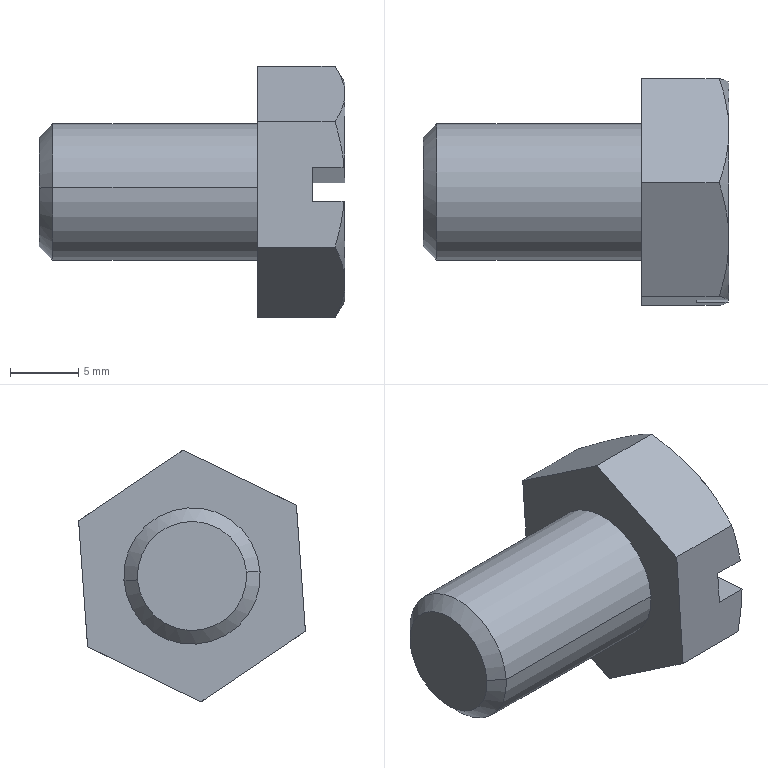Part | SolidWorks | features BaseBody 1 | 1 solid | 23 faces | box 22.4 x 16.618 x 18.428 mm | volume 2560 mm3 | plane 13 | cone 8 | cylinder 2 | commonest cylinder face diameters 10 x2
STEP:
#1=CARTESIAN_POINT('',(442.1,141.01,-29.715));
#2=VERTEX_POINT('',#1);
#3=CARTESIAN_POINT('',(442.1,148.99,-30.285));
#4=VERTEX_POINT('',#3);
#5=CARTESIAN_POINT('',(442.1,145.,-30.));
#6=DIRECTION('',(-1.,0.,0.));
#7=DIRECTION('',(0.,-0.9975,0.07126));
#8=AXIS2_PLACEMENT_3D('',#5,#6,#7);
#9=CIRCLE('',#8,4.);
#10=EDGE_CURVE('',#2,#4,#9,.T.);
#11=ORIENTED_EDGE('',*,*,#10,.F.);
#12=CARTESIAN_POINT('',(443.1,140.013,-29.644));
#13=VERTEX_POINT('',#12);
#14=CARTESIAN_POINT('',(442.1,141.01,-29.715));
#15=DIRECTION('',(0.7071,-0.7053,0.05039));
#16=VECTOR('',#15,1000.);
#17=LINE('',#14,#16);
#18=EDGE_CURVE('',#2,#13,#17,.T.);
#19=ORIENTED_EDGE('',*,*,#18,.T.);
#20=CARTESIAN_POINT('',(443.1,149.987,-30.356));
#21=VERTEX_POINT('',#20);
#22=CARTESIAN_POINT('',(443.1,145.,-30.));
#23=DIRECTION('',(1.,0.,0.));
#24=DIRECTION('',(0.,-0.9975,0.07126));
#25=AXIS2_PLACEMENT_3D('',#22,#23,#24);
#26=CIRCLE('',#25,5.);
#27=EDGE_CURVE('',#21,#13,#26,.T.);
#28=ORIENTED_EDGE('',*,*,#27,.F.);
#29=CARTESIAN_POINT('',(442.1,148.99,-30.285));
#30=DIRECTION('',(0.7071,0.7053,-0.05039));
#31=VECTOR('',#30,1000.);
#32=LINE('',#29,#31);
#33=EDGE_CURVE('',#4,#21,#32,.T.);
#34=ORIENTED_EDGE('',*,*,#33,.F.);
#35=EDGE_LOOP('',(#11,#19,#28,#34));
#36=FACE_OUTER_BOUND('',#35,.T.);
#37=CARTESIAN_POINT('',(442.1,145.,-30.));
#38=DIRECTION('',(1.,0.,0.));
#39=DIRECTION('',(0.,0.9975,-0.07126));
#40=AXIS2_PLACEMENT_3D('',#37,#38,#39);
#41=CONICAL_SURFACE('',#40,4.,0.7854);
#42=ADVANCED_FACE('',(#36),#41,.T.);
#43=ORIENTED_EDGE('',*,*,#27,.T.);
#44=CARTESIAN_POINT('',(458.1,140.013,-29.644));
#45=VERTEX_POINT('',#44);
#46=CARTESIAN_POINT('',(442.1,140.013,-29.644));
#47=DIRECTION('',(1.,0.,0.));
#48=VECTOR('',#47,1000.);
#49=LINE('',#46,#48);
#50=EDGE_CURVE('',#13,#45,#49,.T.);
#51=ORIENTED_EDGE('',*,*,#50,.T.);
#52=CARTESIAN_POINT('',(458.1,149.987,-30.356));
#53=VERTEX_POINT('',#52);
#54=CARTESIAN_POINT('',(458.1,145.,-30.));
#55=DIRECTION('',(-1.,0.,0.));
#56=DIRECTION('',(0.,-0.9975,0.07126));
#57=AXIS2_PLACEMENT_3D('',#54,#55,#56);
#58=CIRCLE('',#57,5.);
#59=EDGE_CURVE('',#45,#53,#58,.T.);
#60=ORIENTED_EDGE('',*,*,#59,.T.);
#61=CARTESIAN_POINT('',(442.1,149.987,-30.356));
#62=DIRECTION('',(1.,0.,0.));
#63=VECTOR('',#62,1000.);
#64=LINE('',#61,#63);
#65=EDGE_CURVE('',#21,#53,#64,.T.);
#66=ORIENTED_EDGE('',*,*,#65,.F.);
#67=EDGE_LOOP('',(#43,#51,#60,#66));
#68=FACE_OUTER_BOUND('',#67,.T.);
#69=CARTESIAN_POINT('',(442.1,145.,-30.));
#70=DIRECTION('',(1.,0.,0.));
#71=DIRECTION('',(0.,0.9975,-0.07126));
#72=AXIS2_PLACEMENT_3D('',#69,#70,#71);
#73=CYLINDRICAL_SURFACE('',#72,5.);
#74=ADVANCED_FACE('',(#68),#73,.T.);
#75=CARTESIAN_POINT('',(458.1,145.658,-20.786));
#76=VERTEX_POINT('',#75);
#77=CARTESIAN_POINT('',(458.1,153.309,-25.963));
#78=VERTEX_POINT('',#77);
#79=CARTESIAN_POINT('',(458.1,153.309,-25.963));
#80=DIRECTION('',(0.,0.8282,-0.5604));
#81=VECTOR('',#80,1000.);
#82=LINE('',#79,#81);
#83=EDGE_CURVE('',#76,#78,#82,.T.);
#84=ORIENTED_EDGE('',*,*,#83,.T.);
#85=CARTESIAN_POINT('',(458.1,152.651,-35.177));
#86=VERTEX_POINT('',#85);
#87=CARTESIAN_POINT('',(458.1,152.651,-35.177));
#88=DIRECTION('',(0.,-0.07126,-0.9975));
#89=VECTOR('',#88,1000.);
#90=LINE('',#87,#89);
#91=EDGE_CURVE('',#78,#86,#90,.T.);
#92=ORIENTED_EDGE('',*,*,#91,.T.);
#93=CARTESIAN_POINT('',(458.1,144.342,-39.214));
#94=VERTEX_POINT('',#93);
#95=CARTESIAN_POINT('',(458.1,152.651,-35.177));
#96=DIRECTION('',(0.,-0.8995,-0.437));
#97=VECTOR('',#96,1000.);
#98=LINE('',#95,#97);
#99=EDGE_CURVE('',#86,#94,#98,.T.);
#100=ORIENTED_EDGE('',*,*,#99,.T.);
#101=CARTESIAN_POINT('',(458.1,136.691,-34.037));
#102=VERTEX_POINT('',#101);
#103=CARTESIAN_POINT('',(458.1,136.691,-34.037));
#104=DIRECTION('',(0.,-0.8282,0.5604));
#105=VECTOR('',#104,1000.);
#106=LINE('',#103,#105);
#107=EDGE_CURVE('',#94,#102,#106,.T.);
#108=ORIENTED_EDGE('',*,*,#107,.T.);
#109=CARTESIAN_POINT('',(458.1,137.349,-24.823));
#110=VERTEX_POINT('',#109);
#111=CARTESIAN_POINT('',(458.1,136.691,-34.037));
#112=DIRECTION('',(0.,0.07126,0.9975));
#113=VECTOR('',#112,1000.);
#114=LINE('',#111,#113);
#115=EDGE_CURVE('',#102,#110,#114,.T.);
#116=ORIENTED_EDGE('',*,*,#115,.T.);
#117=CARTESIAN_POINT('',(458.1,137.349,-24.823));
#118=DIRECTION('',(0.,0.8995,0.437));
#119=VECTOR('',#118,1000.);
#120=LINE('',#117,#119);
#121=EDGE_CURVE('',#110,#76,#120,.T.);
#122=ORIENTED_EDGE('',*,*,#121,.T.);
#123=EDGE_LOOP('',(#84,#92,#100,#108,#116,#122));
#124=FACE_OUTER_BOUND('',#123,.T.);
#125=CARTESIAN_POINT('',(458.1,145.,-30.));
#126=DIRECTION('',(-1.,0.,0.));
#127=DIRECTION('',(0.,-0.9975,0.07126));
#128=AXIS2_PLACEMENT_3D('',#125,#126,#127);
#129=CIRCLE('',#128,5.);
#130=EDGE_CURVE('',#53,#45,#129,.T.);
#131=ORIENTED_EDGE('',*,*,#130,.F.);
#132=ORIENTED_EDGE('',*,*,#59,.F.);
#133=EDGE_LOOP('',(#131,#132));
#134=FACE_BOUND('',#133,.T.);
#135=CARTESIAN_POINT('',(458.1,145.658,-20.786));
#136=DIRECTION('',(-1.,0.,0.));
#137=DIRECTION('',(0.,-0.9975,0.07126));
#138=AXIS2_PLACEMENT_3D('',#135,#136,#137);
#139=PLANE('',#138);
#140=ADVANCED_FACE('',(#124,#134),#139,.T.);
#141=CARTESIAN_POINT('',(464.5,148.496,-37.196));
#142=VERTEX_POINT('',#141);
#143=CARTESIAN_POINT('',(464.5,152.793,-31.81));
#144=VERTEX_POINT('',#143);
#145=CARTESIAN_POINT('',(464.5,145.,-30.));
#146=DIRECTION('',(1.,0.,0.));
#147=DIRECTION('',(0.,0.9975,-0.07126));
#148=AXIS2_PLACEMENT_3D('',#145,#146,#147);
#149=CIRCLE('',#148,8.);
#150=EDGE_CURVE('',#142,#144,#149,.T.);
#151=ORIENTED_EDGE('',*,*,#150,.T.);
#152=CARTESIAN_POINT('',(464.5,137.029,-30.684));
#153=VERTEX_POINT('',#152);
#154=CARTESIAN_POINT('',(464.5,136.931,-30.677));
#155=DIRECTION('',(0.,0.9975,-0.07126));
#156=VECTOR('',#155,1000.);
#157=LINE('',#154,#156);
#158=EDGE_CURVE('',#153,#144,#157,.T.);
#159=ORIENTED_EDGE('',*,*,#158,.F.);
#160=CARTESIAN_POINT('',(464.5,140.516,-36.626));
#161=VERTEX_POINT('',#160);
#162=CARTESIAN_POINT('',(464.5,145.,-30.));
#163=DIRECTION('',(1.,0.,0.));
#164=DIRECTION('',(0.,0.9975,-0.07126));
#165=AXIS2_PLACEMENT_3D('',#162,#163,#164);
#166=CIRCLE('',#165,8.);
#167=EDGE_CURVE('',#153,#161,#166,.T.);
#168=ORIENTED_EDGE('',*,*,#167,.T.);
#169=CARTESIAN_POINT('',(464.5,145.,-30.));
#170=DIRECTION('',(1.,0.,0.));
#171=DIRECTION('',(0.,0.9975,-0.07126));
#172=AXIS2_PLACEMENT_3D('',#169,#170,#171);
#173=CIRCLE('',#172,8.);
#174=EDGE_CURVE('',#161,#142,#173,.T.);
#175=ORIENTED_EDGE('',*,*,#174,.T.);
#176=EDGE_LOOP('',(#151,#159,#168,#175));
#177=FACE_OUTER_BOUND('',#176,.T.);
#178=CARTESIAN_POINT('',(464.5,145.658,-20.786));
#179=DIRECTION('',(-1.,0.,0.));
#180=DIRECTION('',(0.,-0.9975,0.07126));
#181=AXIS2_PLACEMENT_3D('',#178,#179,#180);
#182=PLANE('',#181);
#183=ADVANCED_FACE('',(#177),#182,.F.);
#184=CARTESIAN_POINT('',(463.785,153.309,-25.963));
#185=VERTEX_POINT('',#184);
#186=CARTESIAN_POINT('',(464.5,149.484,-23.374));
#187=VERTEX_POINT('',#186);
#188=CARTESIAN_POINT('',(463.785,153.309,-25.963));
#189=CARTESIAN_POINT('',(464.004,152.683,-25.54));
#190=CARTESIAN_POINT('',(464.183,152.053,-25.113));
#191=CARTESIAN_POINT('',(464.432,150.779,-24.251));
#192=CARTESIAN_POINT('',(464.5,150.135,-23.815));
#193=CARTESIAN_POINT('',(464.5,149.484,-23.374));
#194=B_SPLINE_CURVE_WITH_KNOTS('',3,(#188,#189,#190,#191,#192,#193),.UNSPECIFIED.,.F.,.F.,(4,2,4),(0.000000238,0.002337,0.004674),.UNSPECIFIED.);
#195=EDGE_CURVE('',#185,#187,#194,.T.);
#196=ORIENTED_EDGE('',*,*,#195,.F.);
#197=CARTESIAN_POINT('',(458.1,153.309,-25.963));
#198=DIRECTION('',(1.,0.,0.));
#199=VECTOR('',#198,1000.);
#200=LINE('',#197,#199);
#201=EDGE_CURVE('',#78,#185,#200,.T.);
#202=ORIENTED_EDGE('',*,*,#201,.F.);
#203=ORIENTED_EDGE('',*,*,#83,.F.);
#204=CARTESIAN_POINT('',(463.785,145.658,-20.786));
#205=VERTEX_POINT('',#204);
#206=CARTESIAN_POINT('',(458.1,145.658,-20.786));
#207=DIRECTION('',(1.,0.,0.));
#208=VECTOR('',#207,1000.);
#209=LINE('',#206,#208);
#210=EDGE_CURVE('',#76,#205,#209,.T.);
#211=ORIENTED_EDGE('',*,*,#210,.T.);
#212=CARTESIAN_POINT('',(464.5,149.484,-23.374));
#213=CARTESIAN_POINT('',(464.5,149.159,-23.155));
#214=CARTESIAN_POINT('',(464.483,148.833,-22.934));
#215=CARTESIAN_POINT('',(464.418,148.188,-22.498));
#216=CARTESIAN_POINT('',(464.369,147.867,-22.281));
#217=CARTESIAN_POINT('',(464.183,146.912,-21.634));
#218=CARTESIAN_POINT('',(464.003,146.282,-21.208));
#219=CARTESIAN_POINT('',(463.785,145.658,-20.786));
#220=B_SPLINE_CURVE_WITH_KNOTS('',3,(#212,#213,#214,#215,#216,#217,#218,#219),.UNSPECIFIED.,.F.,.F.,(4,2,2,4),(0.004674,0.005838,0.007002,0.00933),.UNSPECIFIED.);
#221=EDGE_CURVE('',#187,#205,#220,.T.);
#222=ORIENTED_EDGE('',*,*,#221,.F.);
#223=EDGE_LOOP('',(#196,#202,#203,#211,#222));
#224=FACE_OUTER_BOUND('',#223,.T.);
#225=CARTESIAN_POINT('',(458.1,153.309,-25.963));
#226=DIRECTION('',(0.,-0.5604,-0.8282));
#227=DIRECTION('',(0.,-0.8282,0.5604));
#228=AXIS2_PLACEMENT_3D('',#225,#226,#227);
#229=PLANE('',#228);
#230=ADVANCED_FACE('',(#224),#229,.F.);
#231=CARTESIAN_POINT('',(463.785,152.651,-35.177));
#232=VERTEX_POINT('',#231);
#233=CARTESIAN_POINT('',(464.444,152.891,-31.817));
#234=VERTEX_POINT('',#233);
#235=CARTESIAN_POINT('',(463.785,152.651,-35.177));
#236=CARTESIAN_POINT('',(463.945,152.69,-34.628));
#237=CARTESIAN_POINT('',(464.085,152.73,-34.068));
#238=CARTESIAN_POINT('',(464.309,152.81,-32.947));
#239=CARTESIAN_POINT('',(464.393,152.85,-32.383));
#240=CARTESIAN_POINT('',(464.444,152.891,-31.817));
#241=B_SPLINE_CURVE_WITH_KNOTS('',3,(#235,#236,#237,#238,#239,#240),.UNSPECIFIED.,.F.,.F.,(4,2,4),(0.008618,0.01033,0.01204),.UNSPECIFIED.);
#242=EDGE_CURVE('',#232,#234,#241,.T.);
#243=ORIENTED_EDGE('',*,*,#242,.F.);
#244=CARTESIAN_POINT('',(458.1,152.651,-35.177));
#245=DIRECTION('',(1.,0.,0.));
#246=VECTOR('',#245,1000.);
#247=LINE('',#244,#246);
#248=EDGE_CURVE('',#86,#232,#247,.T.);
#249=ORIENTED_EDGE('',*,*,#248,.F.);
#250=ORIENTED_EDGE('',*,*,#91,.F.);
#251=ORIENTED_EDGE('',*,*,#201,.T.);
#252=CARTESIAN_POINT('',(464.444,153.069,-29.323));
#253=VERTEX_POINT('',#252);
#254=CARTESIAN_POINT('',(464.444,153.069,-29.323));
#255=CARTESIAN_POINT('',(464.341,153.151,-28.173));
#256=CARTESIAN_POINT('',(464.102,153.231,-27.058));
#257=CARTESIAN_POINT('',(463.785,153.309,-25.963));
#258=B_SPLINE_CURVE_WITH_KNOTS('',3,(#254,#255,#256,#257),.UNSPECIFIED.,.F.,.F.,(4,4),(0.01454,0.01797),.UNSPECIFIED.);
#259=EDGE_CURVE('',#253,#185,#258,.T.);
#260=ORIENTED_EDGE('',*,*,#259,.F.);
#261=CARTESIAN_POINT('',(462.1,153.069,-29.323));
#262=VERTEX_POINT('',#261);
#263=CARTESIAN_POINT('',(462.1,153.069,-29.323));
#264=DIRECTION('',(1.,0.,0.));
#265=VECTOR('',#264,1000.);
#266=LINE('',#263,#265);
#267=EDGE_CURVE('',#262,#253,#266,.T.);
#268=ORIENTED_EDGE('',*,*,#267,.F.);
#269=CARTESIAN_POINT('',(462.1,152.891,-31.817));
#270=VERTEX_POINT('',#269);
#271=CARTESIAN_POINT('',(462.1,153.069,-29.323));
#272=DIRECTION('',(0.,0.07126,0.9975));
#273=VECTOR('',#272,1000.);
#274=LINE('',#271,#273);
#275=EDGE_CURVE('',#270,#262,#274,.T.);
#276=ORIENTED_EDGE('',*,*,#275,.F.);
#277=CARTESIAN_POINT('',(462.1,152.891,-31.817));
#278=DIRECTION('',(1.,0.,0.));
#279=VECTOR('',#278,1000.);
#280=LINE('',#277,#279);
#281=EDGE_CURVE('',#270,#234,#280,.T.);
#282=ORIENTED_EDGE('',*,*,#281,.T.);
#283=EDGE_LOOP('',(#243,#249,#250,#251,#260,#268,#276,#282));
#284=FACE_OUTER_BOUND('',#283,.T.);
#285=CARTESIAN_POINT('',(458.1,152.651,-35.177));
#286=DIRECTION('',(0.,-0.9975,0.07126));
#287=DIRECTION('',(1.,0.,0.));
#288=AXIS2_PLACEMENT_3D('',#285,#286,#287);
#289=PLANE('',#288);
#290=ADVANCED_FACE('',(#284),#289,.F.);
#291=CARTESIAN_POINT('',(463.785,144.342,-39.214));
#292=VERTEX_POINT('',#291);
#293=CARTESIAN_POINT('',(463.785,144.342,-39.214));
#294=CARTESIAN_POINT('',(464.004,145.021,-38.884));
#295=CARTESIAN_POINT('',(464.183,145.706,-38.551));
#296=CARTESIAN_POINT('',(464.432,147.089,-37.879));
#297=CARTESIAN_POINT('',(464.5,147.788,-37.54));
#298=CARTESIAN_POINT('',(464.5,148.496,-37.196));
#299=B_SPLINE_CURVE_WITH_KNOTS('',3,(#293,#294,#295,#296,#297,#298),.UNSPECIFIED.,.F.,.F.,(4,2,4),(0.000000238,0.002337,0.004674),.UNSPECIFIED.);
#300=EDGE_CURVE('',#292,#142,#299,.T.);
#301=ORIENTED_EDGE('',*,*,#300,.F.);
#302=CARTESIAN_POINT('',(458.1,144.342,-39.214));
#303=DIRECTION('',(1.,0.,0.));
#304=VECTOR('',#303,1000.);
#305=LINE('',#302,#304);
#306=EDGE_CURVE('',#94,#292,#305,.T.);
#307=ORIENTED_EDGE('',*,*,#306,.F.);
#308=ORIENTED_EDGE('',*,*,#99,.F.);
#309=ORIENTED_EDGE('',*,*,#248,.T.);
#310=CARTESIAN_POINT('',(464.5,148.496,-37.196));
#311=CARTESIAN_POINT('',(464.5,148.849,-37.024));
#312=CARTESIAN_POINT('',(464.483,149.203,-36.852));
#313=CARTESIAN_POINT('',(464.418,149.903,-36.512));
#314=CARTESIAN_POINT('',(464.369,150.251,-36.343));
#315=CARTESIAN_POINT('',(464.183,151.289,-35.839));
#316=CARTESIAN_POINT('',(464.003,151.973,-35.507));
#317=CARTESIAN_POINT('',(463.785,152.651,-35.177));
#318=B_SPLINE_CURVE_WITH_KNOTS('',3,(#310,#311,#312,#313,#314,#315,#316,#317),.UNSPECIFIED.,.F.,.F.,(4,2,2,4),(0.004674,0.005838,0.007002,0.00933),.UNSPECIFIED.);
#319=EDGE_CURVE('',#142,#232,#318,.T.);
#320=ORIENTED_EDGE('',*,*,#319,.F.);
#321=EDGE_LOOP('',(#301,#307,#308,#309,#320));
#322=FACE_OUTER_BOUND('',#321,.T.);
#323=CARTESIAN_POINT('',(458.1,152.651,-35.177));
#324=DIRECTION('',(0.,-0.437,0.8995));
#325=DIRECTION('',(0.,0.8995,0.437));
#326=AXIS2_PLACEMENT_3D('',#323,#324,#325);
#327=PLANE('',#326);
#328=ADVANCED_FACE('',(#322),#327,.F.);
#329=CARTESIAN_POINT('',(463.785,136.691,-34.037));
#330=VERTEX_POINT('',#329);
#331=CARTESIAN_POINT('',(463.785,136.691,-34.037));
#332=CARTESIAN_POINT('',(464.004,137.317,-34.46));
#333=CARTESIAN_POINT('',(464.183,137.947,-34.887));
#334=CARTESIAN_POINT('',(464.432,139.221,-35.749));
#335=CARTESIAN_POINT('',(464.5,139.865,-36.185));
#336=CARTESIAN_POINT('',(464.5,140.516,-36.626));
#337=B_SPLINE_CURVE_WITH_KNOTS('',3,(#331,#332,#333,#334,#335,#336),.UNSPECIFIED.,.F.,.F.,(4,2,4),(0.000000238,0.002337,0.004674),.UNSPECIFIED.);
#338=EDGE_CURVE('',#330,#161,#337,.T.);
#339=ORIENTED_EDGE('',*,*,#338,.F.);
#340=CARTESIAN_POINT('',(458.1,136.691,-34.037));
#341=DIRECTION('',(1.,0.,0.));
#342=VECTOR('',#341,1000.);
#343=LINE('',#340,#342);
#344=EDGE_CURVE('',#102,#330,#343,.T.);
#345=ORIENTED_EDGE('',*,*,#344,.F.);
#346=ORIENTED_EDGE('',*,*,#107,.F.);
#347=ORIENTED_EDGE('',*,*,#306,.T.);
#348=CARTESIAN_POINT('',(464.5,140.516,-36.626));
#349=CARTESIAN_POINT('',(464.5,140.841,-36.845));
#350=CARTESIAN_POINT('',(464.483,141.167,-37.066));
#351=CARTESIAN_POINT('',(464.418,141.812,-37.502));
#352=CARTESIAN_POINT('',(464.369,142.133,-37.719));
#353=CARTESIAN_POINT('',(464.183,143.088,-38.366));
#354=CARTESIAN_POINT('',(464.003,143.718,-38.792));
#355=CARTESIAN_POINT('',(463.785,144.342,-39.214));
#356=B_SPLINE_CURVE_WITH_KNOTS('',3,(#348,#349,#350,#351,#352,#353,#354,#355),.UNSPECIFIED.,.F.,.F.,(4,2,2,4),(0.004674,0.005838,0.007002,0.00933),.UNSPECIFIED.);
#357=EDGE_CURVE('',#161,#292,#356,.T.);
#358=ORIENTED_EDGE('',*,*,#357,.F.);
#359=EDGE_LOOP('',(#339,#345,#346,#347,#358));
#360=FACE_OUTER_BOUND('',#359,.T.);
#361=CARTESIAN_POINT('',(458.1,136.691,-34.037));
#362=DIRECTION('',(0.,0.5604,0.8282));
#363=DIRECTION('',(0.,0.8282,-0.5604));
#364=AXIS2_PLACEMENT_3D('',#361,#362,#363);
#365=PLANE('',#364);
#366=ADVANCED_FACE('',(#360),#365,.F.);
#367=CARTESIAN_POINT('',(463.785,137.349,-24.823));
#368=VERTEX_POINT('',#367);
#369=CARTESIAN_POINT('',(464.444,137.109,-28.183));
#370=VERTEX_POINT('',#369);
#371=CARTESIAN_POINT('',(463.785,137.349,-24.823));
#372=CARTESIAN_POINT('',(464.102,137.271,-25.918));
#373=CARTESIAN_POINT('',(464.341,137.192,-27.033));
#374=CARTESIAN_POINT('',(464.444,137.109,-28.183));
#375=B_SPLINE_CURVE_WITH_KNOTS('',3,(#371,#372,#373,#374),.UNSPECIFIED.,.F.,.F.,(4,4),(0.02463,0.02807),.UNSPECIFIED.);
#376=EDGE_CURVE('',#368,#370,#375,.T.);
#377=ORIENTED_EDGE('',*,*,#376,.F.);
#378=CARTESIAN_POINT('',(458.1,137.349,-24.823));
#379=DIRECTION('',(1.,0.,0.));
#380=VECTOR('',#379,1000.);
#381=LINE('',#378,#380);
#382=EDGE_CURVE('',#110,#368,#381,.T.);
#383=ORIENTED_EDGE('',*,*,#382,.F.);
#384=ORIENTED_EDGE('',*,*,#115,.F.);
#385=ORIENTED_EDGE('',*,*,#344,.T.);
#386=CARTESIAN_POINT('',(464.444,136.931,-30.677));
#387=VERTEX_POINT('',#386);
#388=CARTESIAN_POINT('',(464.444,136.931,-30.677));
#389=CARTESIAN_POINT('',(464.393,136.891,-31.243));
#390=CARTESIAN_POINT('',(464.309,136.851,-31.806));
#391=CARTESIAN_POINT('',(464.085,136.77,-32.928));
#392=CARTESIAN_POINT('',(463.945,136.73,-33.487));
#393=CARTESIAN_POINT('',(463.785,136.691,-34.037));
#394=B_SPLINE_CURVE_WITH_KNOTS('',3,(#388,#389,#390,#391,#392,#393),.UNSPECIFIED.,.F.,.F.,(4,2,4),(0.03056,0.03227,0.03398),.UNSPECIFIED.);
#395=EDGE_CURVE('',#387,#330,#394,.T.);
#396=ORIENTED_EDGE('',*,*,#395,.F.);
#397=CARTESIAN_POINT('',(462.1,136.931,-30.677));
#398=VERTEX_POINT('',#397);
#399=CARTESIAN_POINT('',(462.1,136.931,-30.677));
#400=DIRECTION('',(1.,0.,0.));
#401=VECTOR('',#400,1000.);
#402=LINE('',#399,#401);
#403=EDGE_CURVE('',#398,#387,#402,.T.);
#404=ORIENTED_EDGE('',*,*,#403,.F.);
#405=CARTESIAN_POINT('',(462.1,137.109,-28.183));
#406=VERTEX_POINT('',#405);
#407=CARTESIAN_POINT('',(462.1,136.931,-30.677));
#408=DIRECTION('',(0.,-0.07126,-0.9975));
#409=VECTOR('',#408,1000.);
#410=LINE('',#407,#409);
#411=EDGE_CURVE('',#406,#398,#410,.T.);
#412=ORIENTED_EDGE('',*,*,#411,.F.);
#413=CARTESIAN_POINT('',(462.1,137.109,-28.183));
#414=DIRECTION('',(1.,0.,0.));
#415=VECTOR('',#414,1000.);
#416=LINE('',#413,#415);
#417=EDGE_CURVE('',#406,#370,#416,.T.);
#418=ORIENTED_EDGE('',*,*,#417,.T.);
#419=EDGE_LOOP('',(#377,#383,#384,#385,#396,#404,#412,#418));
#420=FACE_OUTER_BOUND('',#419,.T.);
#421=CARTESIAN_POINT('',(458.1,136.691,-34.037));
#422=DIRECTION('',(0.,0.9975,-0.07126));
#423=DIRECTION('',(-1.,0.,0.));
#424=AXIS2_PLACEMENT_3D('',#421,#422,#423);
#425=PLANE('',#424);
#426=ADVANCED_FACE('',(#420),#425,.F.);
#427=CARTESIAN_POINT('',(464.5,141.504,-22.804));
#428=VERTEX_POINT('',#427);
#429=CARTESIAN_POINT('',(463.785,145.658,-20.786));
#430=CARTESIAN_POINT('',(464.004,144.979,-21.116));
#431=CARTESIAN_POINT('',(464.183,144.294,-21.449));
#432=CARTESIAN_POINT('',(464.432,142.911,-22.121));
#433=CARTESIAN_POINT('',(464.5,142.212,-22.46));
#434=CARTESIAN_POINT('',(464.5,141.504,-22.804));
#435=B_SPLINE_CURVE_WITH_KNOTS('',3,(#429,#430,#431,#432,#433,#434),.UNSPECIFIED.,.F.,.F.,(4,2,4),(0.000000238,0.002337,0.004674),.UNSPECIFIED.);
#436=EDGE_CURVE('',#205,#428,#435,.T.);
#437=ORIENTED_EDGE('',*,*,#436,.F.);
#438=ORIENTED_EDGE('',*,*,#210,.F.);
#439=ORIENTED_EDGE('',*,*,#121,.F.);
#440=ORIENTED_EDGE('',*,*,#382,.T.);
#441=CARTESIAN_POINT('',(464.5,141.504,-22.804));
#442=CARTESIAN_POINT('',(464.5,141.151,-22.976));
#443=CARTESIAN_POINT('',(464.483,140.797,-23.148));
#444=CARTESIAN_POINT('',(464.418,140.097,-23.488));
#445=CARTESIAN_POINT('',(464.369,139.749,-23.657));
#446=CARTESIAN_POINT('',(464.183,138.711,-24.161));
#447=CARTESIAN_POINT('',(464.003,138.027,-24.493));
#448=CARTESIAN_POINT('',(463.785,137.349,-24.823));
#449=B_SPLINE_CURVE_WITH_KNOTS('',3,(#441,#442,#443,#444,#445,#446,#447,#448),.UNSPECIFIED.,.F.,.F.,(4,2,2,4),(0.004674,0.005838,0.007002,0.00933),.UNSPECIFIED.);
#450=EDGE_CURVE('',#428,#368,#449,.T.);
#451=ORIENTED_EDGE('',*,*,#450,.F.);
#452=EDGE_LOOP('',(#437,#438,#439,#440,#451));
#453=FACE_OUTER_BOUND('',#452,.T.);
#454=CARTESIAN_POINT('',(458.1,137.349,-24.823));
#455=DIRECTION('',(0.,0.437,-0.8995));
#456=DIRECTION('',(0.,-0.8995,-0.437));
#457=AXIS2_PLACEMENT_3D('',#454,#455,#456);
#458=PLANE('',#457);
#459=ADVANCED_FACE('',(#453),#458,.F.);
#460=CARTESIAN_POINT('',(464.5,137.207,-28.19));
#461=VERTEX_POINT('',#460);
#462=CARTESIAN_POINT('',(464.5,145.,-30.));
#463=DIRECTION('',(1.,0.,0.));
#464=DIRECTION('',(0.,0.9975,-0.07126));
#465=AXIS2_PLACEMENT_3D('',#462,#463,#464);
#466=CIRCLE('',#465,8.);
#467=EDGE_CURVE('',#428,#461,#466,.T.);
#468=ORIENTED_EDGE('',*,*,#467,.T.);
#469=CARTESIAN_POINT('',(464.5,152.971,-29.316));
#470=VERTEX_POINT('',#469);
#471=CARTESIAN_POINT('',(464.5,137.109,-28.183));
#472=DIRECTION('',(0.,-0.9975,0.07126));
#473=VECTOR('',#472,1000.);
#474=LINE('',#471,#473);
#475=EDGE_CURVE('',#470,#461,#474,.T.);
#476=ORIENTED_EDGE('',*,*,#475,.F.);
#477=CARTESIAN_POINT('',(464.5,145.,-30.));
#478=DIRECTION('',(1.,0.,0.));
#479=DIRECTION('',(0.,0.9975,-0.07126));
#480=AXIS2_PLACEMENT_3D('',#477,#478,#479);
#481=CIRCLE('',#480,8.);
#482=EDGE_CURVE('',#470,#187,#481,.T.);
#483=ORIENTED_EDGE('',*,*,#482,.T.);
#484=CARTESIAN_POINT('',(464.5,145.,-30.));
#485=DIRECTION('',(1.,0.,0.));
#486=DIRECTION('',(0.,0.9975,-0.07126));
#487=AXIS2_PLACEMENT_3D('',#484,#485,#486);
#488=CIRCLE('',#487,8.);
#489=EDGE_CURVE('',#187,#428,#488,.T.);
#490=ORIENTED_EDGE('',*,*,#489,.T.);
#491=EDGE_LOOP('',(#468,#476,#483,#490));
#492=FACE_OUTER_BOUND('',#491,.T.);
#493=CARTESIAN_POINT('',(464.5,145.658,-20.786));
#494=DIRECTION('',(-1.,0.,0.));
#495=DIRECTION('',(0.,-0.9975,0.07126));
#496=AXIS2_PLACEMENT_3D('',#493,#494,#495);
#497=PLANE('',#496);
#498=ADVANCED_FACE('',(#492),#497,.F.);
#499=CARTESIAN_POINT('',(464.444,152.891,-31.817));
#500=CARTESIAN_POINT('',(464.463,152.858,-31.815));
#501=CARTESIAN_POINT('',(464.481,152.825,-31.812));
#502=CARTESIAN_POINT('',(464.5,152.793,-31.81));
#503=B_SPLINE_CURVE_WITH_KNOTS('',3,(#499,#500,#501,#502),.UNSPECIFIED.,.F.,.F.,(4,4),(0.01119,0.01131),.UNSPECIFIED.);
#504=EDGE_CURVE('',#234,#144,#503,.T.);
#505=ORIENTED_EDGE('',*,*,#504,.F.);
#506=ORIENTED_EDGE('',*,*,#281,.F.);
#507=CARTESIAN_POINT('',(462.1,136.931,-30.677));
#508=DIRECTION('',(0.,0.9975,-0.07126));
#509=VECTOR('',#508,1000.);
#510=LINE('',#507,#509);
#511=EDGE_CURVE('',#398,#270,#510,.T.);
#512=ORIENTED_EDGE('',*,*,#511,.F.);
#513=ORIENTED_EDGE('',*,*,#403,.T.);
#514=CARTESIAN_POINT('',(464.5,137.029,-30.684));
#515=CARTESIAN_POINT('',(464.481,136.997,-30.681));
#516=CARTESIAN_POINT('',(464.463,136.964,-30.679));
#517=CARTESIAN_POINT('',(464.444,136.931,-30.677));
#518=B_SPLINE_CURVE_WITH_KNOTS('',3,(#514,#515,#516,#517),.UNSPECIFIED.,.F.,.F.,(4,4),(0.02906,0.02918),.UNSPECIFIED.);
#519=EDGE_CURVE('',#153,#387,#518,.T.);
#520=ORIENTED_EDGE('',*,*,#519,.F.);
#521=ORIENTED_EDGE('',*,*,#158,.T.);
#522=EDGE_LOOP('',(#505,#506,#512,#513,#520,#521));
#523=FACE_OUTER_BOUND('',#522,.T.);
#524=CARTESIAN_POINT('',(462.1,136.931,-30.677));
#525=DIRECTION('',(0.,-0.07126,-0.9975));
#526=DIRECTION('',(0.,-0.9975,0.07126));
#527=AXIS2_PLACEMENT_3D('',#524,#525,#526);
#528=PLANE('',#527);
#529=ADVANCED_FACE('',(#523),#528,.F.);
#530=CARTESIAN_POINT('',(464.444,137.109,-28.183));
#531=CARTESIAN_POINT('',(464.463,137.142,-28.185));
#532=CARTESIAN_POINT('',(464.481,137.175,-28.188));
#533=CARTESIAN_POINT('',(464.5,137.207,-28.19));
#534=B_SPLINE_CURVE_WITH_KNOTS('',3,(#530,#531,#532,#533),.UNSPECIFIED.,.F.,.F.,(4,4),(0.01119,0.01131),.UNSPECIFIED.);
#535=EDGE_CURVE('',#370,#461,#534,.T.);
#536=ORIENTED_EDGE('',*,*,#535,.F.);
#537=ORIENTED_EDGE('',*,*,#417,.F.);
#538=CARTESIAN_POINT('',(462.1,137.109,-28.183));
#539=DIRECTION('',(0.,-0.9975,0.07126));
#540=VECTOR('',#539,1000.);
#541=LINE('',#538,#540);
#542=EDGE_CURVE('',#262,#406,#541,.T.);
#543=ORIENTED_EDGE('',*,*,#542,.F.);
#544=ORIENTED_EDGE('',*,*,#267,.T.);
#545=CARTESIAN_POINT('',(464.5,152.971,-29.316));
#546=CARTESIAN_POINT('',(464.481,153.003,-29.319));
#547=CARTESIAN_POINT('',(464.463,153.036,-29.321));
#548=CARTESIAN_POINT('',(464.444,153.069,-29.323));
#549=B_SPLINE_CURVE_WITH_KNOTS('',3,(#545,#546,#547,#548),.UNSPECIFIED.,.F.,.F.,(4,4),(0.02906,0.02918),.UNSPECIFIED.);
#550=EDGE_CURVE('',#470,#253,#549,.T.);
#551=ORIENTED_EDGE('',*,*,#550,.F.);
#552=ORIENTED_EDGE('',*,*,#475,.T.);
#553=EDGE_LOOP('',(#536,#537,#543,#544,#551,#552));
#554=FACE_OUTER_BOUND('',#553,.T.);
#555=CARTESIAN_POINT('',(462.1,137.109,-28.183));
#556=DIRECTION('',(0.,0.07126,0.9975));
#557=DIRECTION('',(0.,0.9975,-0.07126));
#558=AXIS2_PLACEMENT_3D('',#555,#556,#557);
#559=PLANE('',#558);
#560=ADVANCED_FACE('',(#554),#559,.F.);
#561=ORIENTED_EDGE('',*,*,#275,.T.);
#562=ORIENTED_EDGE('',*,*,#542,.T.);
#563=ORIENTED_EDGE('',*,*,#411,.T.);
#564=ORIENTED_EDGE('',*,*,#511,.T.);
#565=EDGE_LOOP('',(#561,#562,#563,#564));
#566=FACE_OUTER_BOUND('',#565,.T.);
#567=CARTESIAN_POINT('',(462.1,152.891,-31.817));
#568=DIRECTION('',(1.,0.,0.));
#569=DIRECTION('',(0.,0.9975,-0.07126));
#570=AXIS2_PLACEMENT_3D('',#567,#568,#569);
#571=PLANE('',#570);
#572=ADVANCED_FACE('',(#566),#571,.T.);
#573=ORIENTED_EDGE('',*,*,#195,.T.);
#574=ORIENTED_EDGE('',*,*,#482,.F.);
#575=ORIENTED_EDGE('',*,*,#550,.T.);
#576=ORIENTED_EDGE('',*,*,#259,.T.);
#577=EDGE_LOOP('',(#573,#574,#575,#576));
#578=FACE_OUTER_BOUND('',#577,.T.);
#579=CARTESIAN_POINT('',(464.5,145.,-30.));
#580=DIRECTION('',(-1.,0.,0.));
#581=DIRECTION('',(0.,0.9975,-0.07126));
#582=AXIS2_PLACEMENT_3D('',#579,#580,#581);
#583=CONICAL_SURFACE('',#582,8.,1.047);
#584=ADVANCED_FACE('',(#578),#583,.T.);
#585=ORIENTED_EDGE('',*,*,#535,.T.);
#586=ORIENTED_EDGE('',*,*,#467,.F.);
#587=ORIENTED_EDGE('',*,*,#450,.T.);
#588=ORIENTED_EDGE('',*,*,#376,.T.);
#589=EDGE_LOOP('',(#585,#586,#587,#588));
#590=FACE_OUTER_BOUND('',#589,.T.);
#591=CARTESIAN_POINT('',(464.5,145.,-30.));
#592=DIRECTION('',(-1.,0.,0.));
#593=DIRECTION('',(0.,0.9975,-0.07126));
#594=AXIS2_PLACEMENT_3D('',#591,#592,#593);
#595=CONICAL_SURFACE('',#594,8.,1.047);
#596=ADVANCED_FACE('',(#590),#595,.T.);
#597=ORIENTED_EDGE('',*,*,#338,.T.);
#598=ORIENTED_EDGE('',*,*,#167,.F.);
#599=ORIENTED_EDGE('',*,*,#519,.T.);
#600=ORIENTED_EDGE('',*,*,#395,.T.);
#601=EDGE_LOOP('',(#597,#598,#599,#600));
#602=FACE_OUTER_BOUND('',#601,.T.);
#603=CARTESIAN_POINT('',(464.5,145.,-30.));
#604=DIRECTION('',(-1.,0.,0.));
#605=DIRECTION('',(0.,0.9975,-0.07126));
#606=AXIS2_PLACEMENT_3D('',#603,#604,#605);
#607=CONICAL_SURFACE('',#606,8.,1.047);
#608=ADVANCED_FACE('',(#602),#607,.T.);
#609=ORIENTED_EDGE('',*,*,#504,.T.);
#610=ORIENTED_EDGE('',*,*,#150,.F.);
#611=ORIENTED_EDGE('',*,*,#319,.T.);
#612=ORIENTED_EDGE('',*,*,#242,.T.);
#613=EDGE_LOOP('',(#609,#610,#611,#612));
#614=FACE_OUTER_BOUND('',#613,.T.);
#615=CARTESIAN_POINT('',(464.5,145.,-30.));
#616=DIRECTION('',(-1.,0.,0.));
#617=DIRECTION('',(0.,0.9975,-0.07126));
#618=AXIS2_PLACEMENT_3D('',#615,#616,#617);
#619=CONICAL_SURFACE('',#618,8.,1.047);
#620=ADVANCED_FACE('',(#614),#619,.T.);
#621=ORIENTED_EDGE('',*,*,#436,.T.);
#622=ORIENTED_EDGE('',*,*,#489,.F.);
#623=ORIENTED_EDGE('',*,*,#221,.T.);
#624=EDGE_LOOP('',(#621,#622,#623));
#625=FACE_OUTER_BOUND('',#624,.T.);
#626=CARTESIAN_POINT('',(464.5,145.,-30.));
#627=DIRECTION('',(-1.,0.,0.));
#628=DIRECTION('',(0.,0.9975,-0.07126));
#629=AXIS2_PLACEMENT_3D('',#626,#627,#628);
#630=CONICAL_SURFACE('',#629,8.,1.047);
#631=ADVANCED_FACE('',(#625),#630,.T.);
#632=ORIENTED_EDGE('',*,*,#300,.T.);
#633=ORIENTED_EDGE('',*,*,#174,.F.);
#634=ORIENTED_EDGE('',*,*,#357,.T.);
#635=EDGE_LOOP('',(#632,#633,#634));
#636=FACE_OUTER_BOUND('',#635,.T.);
#637=CARTESIAN_POINT('',(464.5,145.,-30.));
#638=DIRECTION('',(-1.,0.,0.));
#639=DIRECTION('',(0.,0.9975,-0.07126));
#640=AXIS2_PLACEMENT_3D('',#637,#638,#639);
#641=CONICAL_SURFACE('',#640,8.,1.047);
#642=ADVANCED_FACE('',(#636),#641,.T.);
#643=ORIENTED_EDGE('',*,*,#50,.F.);
#644=CARTESIAN_POINT('',(443.1,145.,-30.));
#645=DIRECTION('',(1.,0.,0.));
#646=DIRECTION('',(0.,-0.9975,0.07126));
#647=AXIS2_PLACEMENT_3D('',#644,#645,#646);
#648=CIRCLE('',#647,5.);
#649=EDGE_CURVE('',#13,#21,#648,.T.);
#650=ORIENTED_EDGE('',*,*,#649,.T.);
#651=ORIENTED_EDGE('',*,*,#65,.T.);
#652=ORIENTED_EDGE('',*,*,#130,.T.);
#653=EDGE_LOOP('',(#643,#650,#651,#652));
#654=FACE_OUTER_BOUND('',#653,.T.);
#655=CARTESIAN_POINT('',(442.1,145.,-30.));
#656=DIRECTION('',(1.,0.,0.));
#657=DIRECTION('',(0.,0.9975,-0.07126));
#658=AXIS2_PLACEMENT_3D('',#655,#656,#657);
#659=CYLINDRICAL_SURFACE('',#658,5.);
#660=ADVANCED_FACE('',(#654),#659,.T.);
#661=CARTESIAN_POINT('',(442.1,145.,-30.));
#662=DIRECTION('',(-1.,0.,0.));
#663=DIRECTION('',(0.,-0.9975,0.07126));
#664=AXIS2_PLACEMENT_3D('',#661,#662,#663);
#665=CIRCLE('',#664,4.);
#666=EDGE_CURVE('',#4,#2,#665,.T.);
#667=ORIENTED_EDGE('',*,*,#666,.T.);
#668=ORIENTED_EDGE('',*,*,#10,.T.);
#669=EDGE_LOOP('',(#667,#668));
#670=FACE_OUTER_BOUND('',#669,.T.);
#671=CARTESIAN_POINT('',(442.1,145.,-30.));
#672=DIRECTION('',(-1.,0.,0.));
#673=DIRECTION('',(0.,-0.9975,0.07126));
#674=AXIS2_PLACEMENT_3D('',#671,#672,#673);
#675=PLANE('',#674);
#676=ADVANCED_FACE('',(#670),#675,.T.);
#677=ORIENTED_EDGE('',*,*,#18,.F.);
#678=ORIENTED_EDGE('',*,*,#666,.F.);
#679=ORIENTED_EDGE('',*,*,#33,.T.);
#680=ORIENTED_EDGE('',*,*,#649,.F.);
#681=EDGE_LOOP('',(#677,#678,#679,#680));
#682=FACE_OUTER_BOUND('',#681,.T.);
#683=CARTESIAN_POINT('',(442.1,145.,-30.));
#684=DIRECTION('',(1.,0.,0.));
#685=DIRECTION('',(0.,0.9975,-0.07126));
#686=AXIS2_PLACEMENT_3D('',#683,#684,#685);
#687=CONICAL_SURFACE('',#686,4.,0.7854);
#688=ADVANCED_FACE('',(#682),#687,.T.);
#689=CLOSED_SHELL('',(#42,#74,#140,#183,#230,#290,#328,#366,#426,#459,#498,#529,#560,#572,#584,#596,#608,#620,#631,#642,#660,#676,#688));
#690=MANIFOLD_SOLID_BREP('',#689);
#691=CARTESIAN_POINT('',(0.,0.,0.));
#692=DIRECTION('',(0.,0.,1.));
#693=DIRECTION('',(1.,0.,0.));
#694=AXIS2_PLACEMENT_3D('',#691,#692,#693);
#695=(LENGTH_UNIT()NAMED_UNIT(*)SI_UNIT(.MILLI.,.METRE.));
#696=UNCERTAINTY_MEASURE_WITH_UNIT(LENGTH_MEASURE(0.00001),#695,'','');
#697=(NAMED_UNIT(*)PLANE_ANGLE_UNIT()SI_UNIT($,.RADIAN.));
#698=(NAMED_UNIT(*)SI_UNIT($,.STERADIAN.)SOLID_ANGLE_UNIT());
#699=(GEOMETRIC_REPRESENTATION_CONTEXT(3)GLOBAL_UNCERTAINTY_ASSIGNED_CONTEXT((#696))GLOBAL_UNIT_ASSIGNED_CONTEXT((#695,#697,#698))REPRESENTATION_CONTEXT('',''));
#700=ADVANCED_BREP_SHAPE_REPRESENTATION('',(#690,#694),#699);